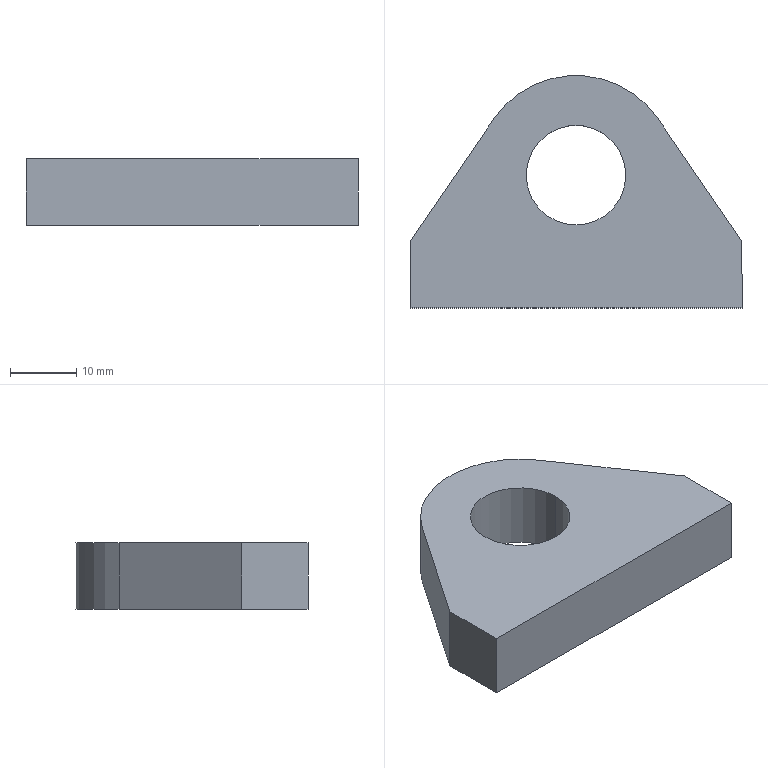Part | SolidWorks | features Extrusion 1 | 1 solid | 10 faces | box 50 x 35 x 10 mm | volume 11273 mm3 | plane 7 | cylinder 3 | commonest cylinder face diameters 15 x2 30 x1
STEP:
#1=CARTESIAN_POINT('',(-7.5,0.,10.));
#2=VERTEX_POINT('',#1);
#3=CARTESIAN_POINT('',(7.5,0.,10.));
#4=VERTEX_POINT('',#3);
#5=CARTESIAN_POINT('',(0.,0.,10.));
#6=DIRECTION('',(0.,0.,1.));
#7=DIRECTION('',(1.,0.,0.));
#8=AXIS2_PLACEMENT_3D('',#5,#6,#7);
#9=CIRCLE('',#8,7.5);
#10=EDGE_CURVE('',#2,#4,#9,.T.);
#11=ORIENTED_EDGE('',*,*,#10,.T.);
#12=CARTESIAN_POINT('',(7.5,0.,0.));
#13=VERTEX_POINT('',#12);
#14=CARTESIAN_POINT('',(7.5,0.,10.));
#15=DIRECTION('',(0.,0.,-1.));
#16=VECTOR('',#15,1000.);
#17=LINE('',#14,#16);
#18=EDGE_CURVE('',#4,#13,#17,.T.);
#19=ORIENTED_EDGE('',*,*,#18,.T.);
#20=CARTESIAN_POINT('',(-7.5,0.,0.));
#21=VERTEX_POINT('',#20);
#22=CARTESIAN_POINT('',(0.,0.,0.));
#23=DIRECTION('',(0.,0.,1.));
#24=DIRECTION('',(1.,0.,0.));
#25=AXIS2_PLACEMENT_3D('',#22,#23,#24);
#26=CIRCLE('',#25,7.5);
#27=EDGE_CURVE('',#21,#13,#26,.T.);
#28=ORIENTED_EDGE('',*,*,#27,.F.);
#29=CARTESIAN_POINT('',(-7.5,0.,10.));
#30=DIRECTION('',(0.,0.,-1.));
#31=VECTOR('',#30,1000.);
#32=LINE('',#29,#31);
#33=EDGE_CURVE('',#2,#21,#32,.T.);
#34=ORIENTED_EDGE('',*,*,#33,.F.);
#35=EDGE_LOOP('',(#11,#19,#28,#34));
#36=FACE_OUTER_BOUND('',#35,.T.);
#37=CARTESIAN_POINT('',(0.,0.,10.));
#38=DIRECTION('',(0.,0.,-1.));
#39=DIRECTION('',(-1.,0.,0.));
#40=AXIS2_PLACEMENT_3D('',#37,#38,#39);
#41=CYLINDRICAL_SURFACE('',#40,7.5);
#42=ADVANCED_FACE('',(#36),#41,.F.);
#43=CARTESIAN_POINT('',(25.,-20.,10.));
#44=VERTEX_POINT('',#43);
#45=CARTESIAN_POINT('',(25.,-10.,10.));
#46=VERTEX_POINT('',#45);
#47=CARTESIAN_POINT('',(25.,-20.,10.));
#48=DIRECTION('',(0.,1.,0.));
#49=VECTOR('',#48,1000.);
#50=LINE('',#47,#49);
#51=EDGE_CURVE('',#44,#46,#50,.T.);
#52=ORIENTED_EDGE('',*,*,#51,.T.);
#53=CARTESIAN_POINT('',(12.385,8.462,10.));
#54=VERTEX_POINT('',#53);
#55=CARTESIAN_POINT('',(25.,-10.,10.));
#56=DIRECTION('',(-0.5642,0.8257,0.));
#57=VECTOR('',#56,1000.);
#58=LINE('',#55,#57);
#59=EDGE_CURVE('',#46,#54,#58,.T.);
#60=ORIENTED_EDGE('',*,*,#59,.T.);
#61=CARTESIAN_POINT('',(-12.385,8.462,10.));
#62=VERTEX_POINT('',#61);
#63=CARTESIAN_POINT('',(0.,0.,10.));
#64=DIRECTION('',(0.,0.,1.));
#65=DIRECTION('',(1.,0.,0.));
#66=AXIS2_PLACEMENT_3D('',#63,#64,#65);
#67=CIRCLE('',#66,15.);
#68=EDGE_CURVE('',#54,#62,#67,.T.);
#69=ORIENTED_EDGE('',*,*,#68,.T.);
#70=CARTESIAN_POINT('',(-25.,-10.,10.));
#71=VERTEX_POINT('',#70);
#72=CARTESIAN_POINT('',(-25.,-10.,10.));
#73=DIRECTION('',(-0.5642,-0.8257,0.));
#74=VECTOR('',#73,1000.);
#75=LINE('',#72,#74);
#76=EDGE_CURVE('',#62,#71,#75,.T.);
#77=ORIENTED_EDGE('',*,*,#76,.T.);
#78=CARTESIAN_POINT('',(-25.,-20.,10.));
#79=VERTEX_POINT('',#78);
#80=CARTESIAN_POINT('',(-25.,-20.,10.));
#81=DIRECTION('',(0.,-1.,0.));
#82=VECTOR('',#81,1000.);
#83=LINE('',#80,#82);
#84=EDGE_CURVE('',#71,#79,#83,.T.);
#85=ORIENTED_EDGE('',*,*,#84,.T.);
#86=CARTESIAN_POINT('',(25.,-20.,10.));
#87=DIRECTION('',(1.,0.,0.));
#88=VECTOR('',#87,1000.);
#89=LINE('',#86,#88);
#90=EDGE_CURVE('',#79,#44,#89,.T.);
#91=ORIENTED_EDGE('',*,*,#90,.T.);
#92=EDGE_LOOP('',(#52,#60,#69,#77,#85,#91));
#93=FACE_OUTER_BOUND('',#92,.T.);
#94=ORIENTED_EDGE('',*,*,#10,.F.);
#95=CARTESIAN_POINT('',(0.,0.,10.));
#96=DIRECTION('',(0.,0.,1.));
#97=DIRECTION('',(1.,0.,0.));
#98=AXIS2_PLACEMENT_3D('',#95,#96,#97);
#99=CIRCLE('',#98,7.5);
#100=EDGE_CURVE('',#4,#2,#99,.T.);
#101=ORIENTED_EDGE('',*,*,#100,.F.);
#102=EDGE_LOOP('',(#94,#101));
#103=FACE_BOUND('',#102,.T.);
#104=CARTESIAN_POINT('',(0.,0.,10.));
#105=DIRECTION('',(0.,0.,1.));
#106=DIRECTION('',(1.,0.,0.));
#107=AXIS2_PLACEMENT_3D('',#104,#105,#106);
#108=PLANE('',#107);
#109=ADVANCED_FACE('',(#93,#103),#108,.T.);
#110=CARTESIAN_POINT('',(25.,-20.,0.));
#111=VERTEX_POINT('',#110);
#112=CARTESIAN_POINT('',(25.,-10.,0.));
#113=VERTEX_POINT('',#112);
#114=CARTESIAN_POINT('',(25.,-20.,0.));
#115=DIRECTION('',(0.,1.,0.));
#116=VECTOR('',#115,1000.);
#117=LINE('',#114,#116);
#118=EDGE_CURVE('',#111,#113,#117,.T.);
#119=ORIENTED_EDGE('',*,*,#118,.F.);
#120=CARTESIAN_POINT('',(-25.,-20.,0.));
#121=VERTEX_POINT('',#120);
#122=CARTESIAN_POINT('',(25.,-20.,0.));
#123=DIRECTION('',(1.,0.,0.));
#124=VECTOR('',#123,1000.);
#125=LINE('',#122,#124);
#126=EDGE_CURVE('',#121,#111,#125,.T.);
#127=ORIENTED_EDGE('',*,*,#126,.F.);
#128=CARTESIAN_POINT('',(-25.,-10.,0.));
#129=VERTEX_POINT('',#128);
#130=CARTESIAN_POINT('',(-25.,-20.,0.));
#131=DIRECTION('',(0.,-1.,0.));
#132=VECTOR('',#131,1000.);
#133=LINE('',#130,#132);
#134=EDGE_CURVE('',#129,#121,#133,.T.);
#135=ORIENTED_EDGE('',*,*,#134,.F.);
#136=CARTESIAN_POINT('',(-12.385,8.462,0.));
#137=VERTEX_POINT('',#136);
#138=CARTESIAN_POINT('',(-25.,-10.,0.));
#139=DIRECTION('',(-0.5642,-0.8257,0.));
#140=VECTOR('',#139,1000.);
#141=LINE('',#138,#140);
#142=EDGE_CURVE('',#137,#129,#141,.T.);
#143=ORIENTED_EDGE('',*,*,#142,.F.);
#144=CARTESIAN_POINT('',(12.385,8.462,0.));
#145=VERTEX_POINT('',#144);
#146=CARTESIAN_POINT('',(0.,0.,0.));
#147=DIRECTION('',(0.,0.,1.));
#148=DIRECTION('',(1.,0.,0.));
#149=AXIS2_PLACEMENT_3D('',#146,#147,#148);
#150=CIRCLE('',#149,15.);
#151=EDGE_CURVE('',#145,#137,#150,.T.);
#152=ORIENTED_EDGE('',*,*,#151,.F.);
#153=CARTESIAN_POINT('',(25.,-10.,0.));
#154=DIRECTION('',(-0.5642,0.8257,0.));
#155=VECTOR('',#154,1000.);
#156=LINE('',#153,#155);
#157=EDGE_CURVE('',#113,#145,#156,.T.);
#158=ORIENTED_EDGE('',*,*,#157,.F.);
#159=EDGE_LOOP('',(#119,#127,#135,#143,#152,#158));
#160=FACE_OUTER_BOUND('',#159,.T.);
#161=ORIENTED_EDGE('',*,*,#27,.T.);
#162=CARTESIAN_POINT('',(0.,0.,0.));
#163=DIRECTION('',(0.,0.,1.));
#164=DIRECTION('',(1.,0.,0.));
#165=AXIS2_PLACEMENT_3D('',#162,#163,#164);
#166=CIRCLE('',#165,7.5);
#167=EDGE_CURVE('',#13,#21,#166,.T.);
#168=ORIENTED_EDGE('',*,*,#167,.T.);
#169=EDGE_LOOP('',(#161,#168));
#170=FACE_BOUND('',#169,.T.);
#171=CARTESIAN_POINT('',(0.,0.,0.));
#172=DIRECTION('',(0.,0.,1.));
#173=DIRECTION('',(1.,0.,0.));
#174=AXIS2_PLACEMENT_3D('',#171,#172,#173);
#175=PLANE('',#174);
#176=ADVANCED_FACE('',(#160,#170),#175,.F.);
#177=ORIENTED_EDGE('',*,*,#118,.T.);
#178=CARTESIAN_POINT('',(25.,-10.,10.));
#179=DIRECTION('',(0.,0.,-1.));
#180=VECTOR('',#179,1000.);
#181=LINE('',#178,#180);
#182=EDGE_CURVE('',#46,#113,#181,.T.);
#183=ORIENTED_EDGE('',*,*,#182,.F.);
#184=ORIENTED_EDGE('',*,*,#51,.F.);
#185=CARTESIAN_POINT('',(25.,-20.,10.));
#186=DIRECTION('',(0.,0.,-1.));
#187=VECTOR('',#186,1000.);
#188=LINE('',#185,#187);
#189=EDGE_CURVE('',#44,#111,#188,.T.);
#190=ORIENTED_EDGE('',*,*,#189,.T.);
#191=EDGE_LOOP('',(#177,#183,#184,#190));
#192=FACE_OUTER_BOUND('',#191,.T.);
#193=CARTESIAN_POINT('',(25.,-20.,10.));
#194=DIRECTION('',(-1.,0.,0.));
#195=DIRECTION('',(0.,-1.,0.));
#196=AXIS2_PLACEMENT_3D('',#193,#194,#195);
#197=PLANE('',#196);
#198=ADVANCED_FACE('',(#192),#197,.F.);
#199=ORIENTED_EDGE('',*,*,#157,.T.);
#200=CARTESIAN_POINT('',(12.385,8.462,10.));
#201=DIRECTION('',(0.,0.,-1.));
#202=VECTOR('',#201,1000.);
#203=LINE('',#200,#202);
#204=EDGE_CURVE('',#54,#145,#203,.T.);
#205=ORIENTED_EDGE('',*,*,#204,.F.);
#206=ORIENTED_EDGE('',*,*,#59,.F.);
#207=ORIENTED_EDGE('',*,*,#182,.T.);
#208=EDGE_LOOP('',(#199,#205,#206,#207));
#209=FACE_OUTER_BOUND('',#208,.T.);
#210=CARTESIAN_POINT('',(25.,-10.,10.));
#211=DIRECTION('',(-0.8257,-0.5642,0.));
#212=DIRECTION('',(0.5642,-0.8257,0.));
#213=AXIS2_PLACEMENT_3D('',#210,#211,#212);
#214=PLANE('',#213);
#215=ADVANCED_FACE('',(#209),#214,.F.);
#216=ORIENTED_EDGE('',*,*,#151,.T.);
#217=CARTESIAN_POINT('',(-12.385,8.462,10.));
#218=DIRECTION('',(0.,0.,-1.));
#219=VECTOR('',#218,1000.);
#220=LINE('',#217,#219);
#221=EDGE_CURVE('',#62,#137,#220,.T.);
#222=ORIENTED_EDGE('',*,*,#221,.F.);
#223=ORIENTED_EDGE('',*,*,#68,.F.);
#224=ORIENTED_EDGE('',*,*,#204,.T.);
#225=EDGE_LOOP('',(#216,#222,#223,#224));
#226=FACE_OUTER_BOUND('',#225,.T.);
#227=CARTESIAN_POINT('',(0.,0.,10.));
#228=DIRECTION('',(0.,0.,-1.));
#229=DIRECTION('',(-1.,0.,0.));
#230=AXIS2_PLACEMENT_3D('',#227,#228,#229);
#231=CYLINDRICAL_SURFACE('',#230,15.);
#232=ADVANCED_FACE('',(#226),#231,.T.);
#233=ORIENTED_EDGE('',*,*,#142,.T.);
#234=CARTESIAN_POINT('',(-25.,-10.,10.));
#235=DIRECTION('',(0.,0.,-1.));
#236=VECTOR('',#235,1000.);
#237=LINE('',#234,#236);
#238=EDGE_CURVE('',#71,#129,#237,.T.);
#239=ORIENTED_EDGE('',*,*,#238,.F.);
#240=ORIENTED_EDGE('',*,*,#76,.F.);
#241=ORIENTED_EDGE('',*,*,#221,.T.);
#242=EDGE_LOOP('',(#233,#239,#240,#241));
#243=FACE_OUTER_BOUND('',#242,.T.);
#244=CARTESIAN_POINT('',(-25.,-10.,10.));
#245=DIRECTION('',(0.8257,-0.5642,0.));
#246=DIRECTION('',(0.5642,0.8257,0.));
#247=AXIS2_PLACEMENT_3D('',#244,#245,#246);
#248=PLANE('',#247);
#249=ADVANCED_FACE('',(#243),#248,.F.);
#250=ORIENTED_EDGE('',*,*,#134,.T.);
#251=CARTESIAN_POINT('',(-25.,-20.,10.));
#252=DIRECTION('',(0.,0.,-1.));
#253=VECTOR('',#252,1000.);
#254=LINE('',#251,#253);
#255=EDGE_CURVE('',#79,#121,#254,.T.);
#256=ORIENTED_EDGE('',*,*,#255,.F.);
#257=ORIENTED_EDGE('',*,*,#84,.F.);
#258=ORIENTED_EDGE('',*,*,#238,.T.);
#259=EDGE_LOOP('',(#250,#256,#257,#258));
#260=FACE_OUTER_BOUND('',#259,.T.);
#261=CARTESIAN_POINT('',(-25.,-20.,10.));
#262=DIRECTION('',(1.,0.,0.));
#263=DIRECTION('',(0.,0.,-1.));
#264=AXIS2_PLACEMENT_3D('',#261,#262,#263);
#265=PLANE('',#264);
#266=ADVANCED_FACE('',(#260),#265,.F.);
#267=ORIENTED_EDGE('',*,*,#126,.T.);
#268=ORIENTED_EDGE('',*,*,#189,.F.);
#269=ORIENTED_EDGE('',*,*,#90,.F.);
#270=ORIENTED_EDGE('',*,*,#255,.T.);
#271=EDGE_LOOP('',(#267,#268,#269,#270));
#272=FACE_OUTER_BOUND('',#271,.T.);
#273=CARTESIAN_POINT('',(25.,-20.,10.));
#274=DIRECTION('',(0.,1.,0.));
#275=DIRECTION('',(-1.,0.,0.));
#276=AXIS2_PLACEMENT_3D('',#273,#274,#275);
#277=PLANE('',#276);
#278=ADVANCED_FACE('',(#272),#277,.F.);
#279=ORIENTED_EDGE('',*,*,#18,.F.);
#280=ORIENTED_EDGE('',*,*,#100,.T.);
#281=ORIENTED_EDGE('',*,*,#33,.T.);
#282=ORIENTED_EDGE('',*,*,#167,.F.);
#283=EDGE_LOOP('',(#279,#280,#281,#282));
#284=FACE_OUTER_BOUND('',#283,.T.);
#285=CARTESIAN_POINT('',(0.,0.,10.));
#286=DIRECTION('',(0.,0.,-1.));
#287=DIRECTION('',(-1.,0.,0.));
#288=AXIS2_PLACEMENT_3D('',#285,#286,#287);
#289=CYLINDRICAL_SURFACE('',#288,7.5);
#290=ADVANCED_FACE('',(#284),#289,.F.);
#291=CLOSED_SHELL('',(#42,#109,#176,#198,#215,#232,#249,#266,#278,#290));
#292=MANIFOLD_SOLID_BREP('',#291);
#293=CARTESIAN_POINT('',(0.,0.,0.));
#294=DIRECTION('',(0.,0.,1.));
#295=DIRECTION('',(1.,0.,0.));
#296=AXIS2_PLACEMENT_3D('',#293,#294,#295);
#297=(LENGTH_UNIT()NAMED_UNIT(*)SI_UNIT(.MILLI.,.METRE.));
#298=UNCERTAINTY_MEASURE_WITH_UNIT(LENGTH_MEASURE(0.00001),#297,'','');
#299=(NAMED_UNIT(*)PLANE_ANGLE_UNIT()SI_UNIT($,.RADIAN.));
#300=(NAMED_UNIT(*)SI_UNIT($,.STERADIAN.)SOLID_ANGLE_UNIT());
#301=(GEOMETRIC_REPRESENTATION_CONTEXT(3)GLOBAL_UNCERTAINTY_ASSIGNED_CONTEXT((#298))GLOBAL_UNIT_ASSIGNED_CONTEXT((#297,#299,#300))REPRESENTATION_CONTEXT('',''));
#302=ADVANCED_BREP_SHAPE_REPRESENTATION('',(#292,#296),#301);